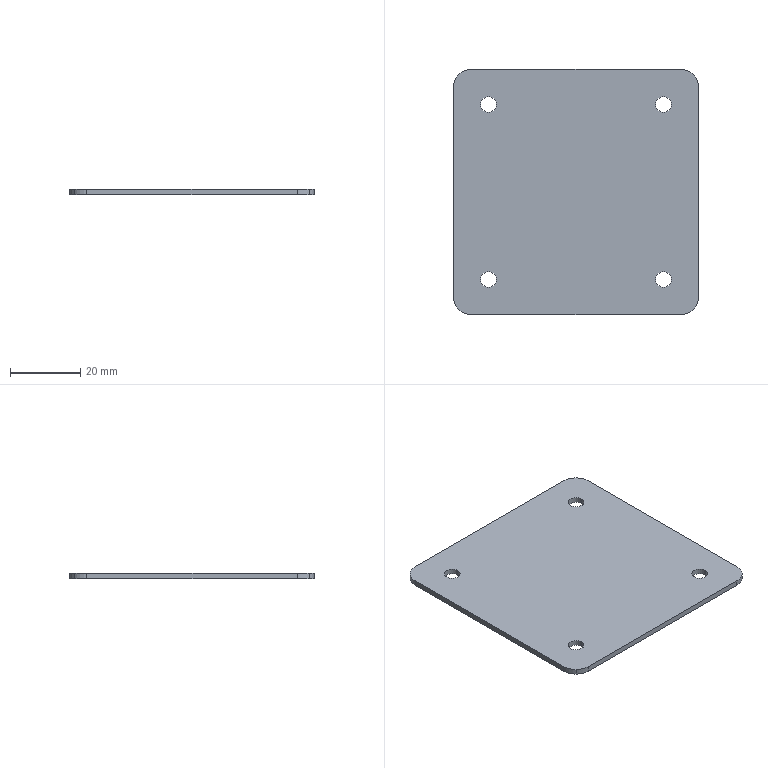Part | STEP file | DCV-000-037 | 1 solid | 22 faces | box 70 x 70 x 1.6 mm | volume 7704 mm3 | cylinder 16 | plane 6 | commonest cylinder face diameters 4.5 x8 10 x8